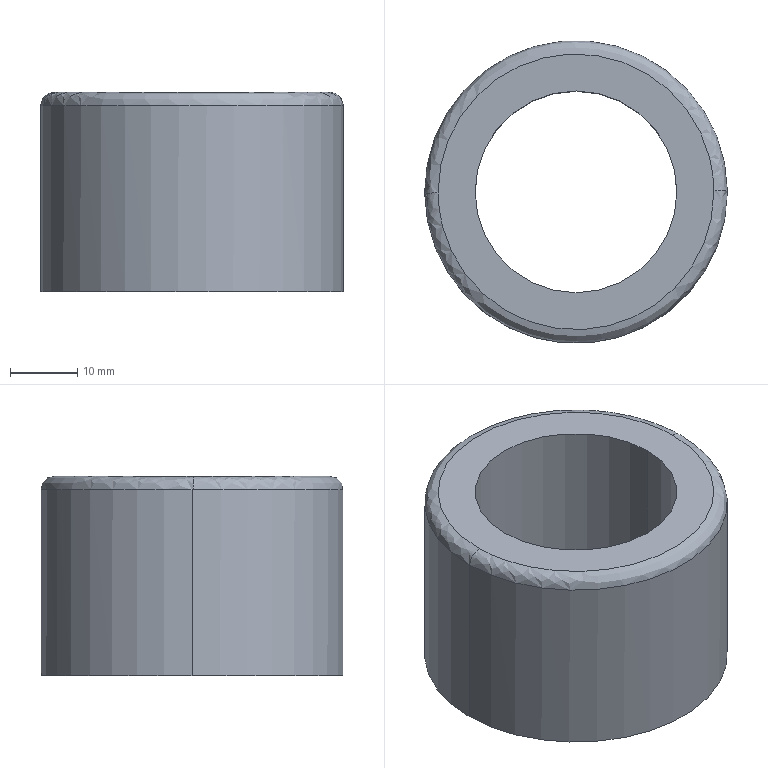Part | SolidWorks | features BaseBody 1 | 1 solid | 8 faces | box 45 x 45 x 29.661 mm | volume 26090 mm3 | cylinder 4 | spline 2 | plane 2 | commonest cylinder face diameters 30 x2 45 x2
STEP:
#1=CARTESIAN_POINT('',(570.036,38.186,21.432));
#2=VERTEX_POINT('',#1);
#3=CARTESIAN_POINT('',(611.034,38.513,21.432));
#4=VERTEX_POINT('',#3);
#5=CARTESIAN_POINT('',(570.036,38.186,21.432));
#6=CARTESIAN_POINT('',(569.708,79.184,21.432));
#7=CARTESIAN_POINT('',(610.707,79.512,21.432));
#8=CARTESIAN_POINT('',(611.034,38.513,21.432));
#9=(BOUNDED_CURVE()B_SPLINE_CURVE(3,(#5,#6,#7,#8),.UNSPECIFIED.,.F.,.T.)B_SPLINE_CURVE_WITH_KNOTS((4,4),(0.,1.),.UNSPECIFIED.)CURVE()GEOMETRIC_REPRESENTATION_ITEM()RATIONAL_B_SPLINE_CURVE((1.,0.3333,0.3333,1.))REPRESENTATION_ITEM(''));
#10=EDGE_CURVE('',#2,#4,#9,.T.);
#11=ORIENTED_EDGE('',*,*,#10,.T.);
#12=CARTESIAN_POINT('',(613.034,38.529,19.432));
#13=VERTEX_POINT('',#12);
#14=CARTESIAN_POINT('',(611.034,38.513,19.432));
#15=DIRECTION('',(-0.007996,1.,0.));
#16=DIRECTION('',(1.,0.007996,-0.000000013));
#17=AXIS2_PLACEMENT_3D('',#14,#15,#16);
#18=CIRCLE('',#17,2.);
#19=EDGE_CURVE('',#4,#13,#18,.T.);
#20=ORIENTED_EDGE('',*,*,#19,.T.);
#21=CARTESIAN_POINT('',(568.035,38.349,19.432));
#22=VERTEX_POINT('',#21);
#23=CARTESIAN_POINT('',(590.535,38.349,19.432));
#24=DIRECTION('',(-0.000000013,0.,-1.));
#25=DIRECTION('',(1.,0.,-0.000000013));
#26=AXIS2_PLACEMENT_3D('',#23,#24,#25);
#27=CIRCLE('',#26,22.5);
#28=EDGE_CURVE('',#22,#13,#27,.T.);
#29=ORIENTED_EDGE('',*,*,#28,.F.);
#30=CARTESIAN_POINT('',(568.036,38.17,19.432));
#31=VERTEX_POINT('',#30);
#32=CARTESIAN_POINT('',(590.535,38.349,19.432));
#33=DIRECTION('',(-0.000000013,0.,-1.));
#34=DIRECTION('',(1.,0.,-0.000000013));
#35=AXIS2_PLACEMENT_3D('',#32,#33,#34);
#36=CIRCLE('',#35,22.5);
#37=EDGE_CURVE('',#31,#22,#36,.T.);
#38=ORIENTED_EDGE('',*,*,#37,.F.);
#39=CARTESIAN_POINT('',(570.036,38.186,19.432));
#40=DIRECTION('',(0.007996,-1.,0.));
#41=DIRECTION('',(-1.,-0.007996,0.000000013));
#42=AXIS2_PLACEMENT_3D('',#39,#40,#41);
#43=CIRCLE('',#42,2.);
#44=EDGE_CURVE('',#2,#31,#43,.T.);
#45=ORIENTED_EDGE('',*,*,#44,.F.);
#46=EDGE_LOOP('',(#11,#20,#29,#38,#45));
#47=FACE_OUTER_BOUND('',#46,.T.);
#48=CARTESIAN_POINT('',(611.034,38.513,21.432));
#49=CARTESIAN_POINT('',(610.707,79.512,21.432));
#50=CARTESIAN_POINT('',(569.708,79.184,21.432));
#51=CARTESIAN_POINT('',(570.036,38.186,21.432));
#52=CARTESIAN_POINT('',(612.206,38.523,21.432));
#53=CARTESIAN_POINT('',(611.859,81.864,21.432));
#54=CARTESIAN_POINT('',(568.518,81.518,21.432));
#55=CARTESIAN_POINT('',(568.864,38.176,21.432));
#56=CARTESIAN_POINT('',(613.034,38.529,20.604));
#57=CARTESIAN_POINT('',(612.675,83.528,20.604));
#58=CARTESIAN_POINT('',(567.676,83.168,20.604));
#59=CARTESIAN_POINT('',(568.036,38.17,20.604));
#60=CARTESIAN_POINT('',(613.034,38.529,19.432));
#61=CARTESIAN_POINT('',(612.675,83.528,19.432));
#62=CARTESIAN_POINT('',(567.676,83.168,19.432));
#63=CARTESIAN_POINT('',(568.036,38.17,19.432));
#64=(BOUNDED_SURFACE()B_SPLINE_SURFACE(3,3,((#48,#49,#50,#51),(#52,#53,#54,#55),(#56,#57,#58,#59),(#60,#61,#62,#63)),.UNSPECIFIED.,.F.,.F.,.F.)B_SPLINE_SURFACE_WITH_KNOTS((4,4),(4,4),(0.,1.),(0.,1.),.UNSPECIFIED.)GEOMETRIC_REPRESENTATION_ITEM()RATIONAL_B_SPLINE_SURFACE(((1.,0.3333,0.3333,1.),(0.8047,0.2682,0.2682,0.8047),(0.8047,0.2682,0.2682,0.8047),(1.,0.3333,0.3333,1.)))REPRESENTATION_ITEM('')SURFACE());
#65=ADVANCED_FACE('',(#47),#64,.T.);
#66=CARTESIAN_POINT('',(613.035,38.349,-8.23));
#67=VERTEX_POINT('',#66);
#68=CARTESIAN_POINT('',(568.035,38.349,-8.23));
#69=VERTEX_POINT('',#68);
#70=CARTESIAN_POINT('',(590.535,38.349,-8.23));
#71=DIRECTION('',(0.000000013,0.,1.));
#72=DIRECTION('',(1.,0.,-0.000000013));
#73=AXIS2_PLACEMENT_3D('',#70,#71,#72);
#74=CIRCLE('',#73,22.5);
#75=EDGE_CURVE('',#67,#69,#74,.T.);
#76=ORIENTED_EDGE('',*,*,#75,.T.);
#77=CARTESIAN_POINT('',(568.035,38.349,6.601));
#78=DIRECTION('',(0.000000013,0.,1.));
#79=VECTOR('',#78,1000.);
#80=LINE('',#77,#79);
#81=EDGE_CURVE('',#69,#22,#80,.T.);
#82=ORIENTED_EDGE('',*,*,#81,.T.);
#83=ORIENTED_EDGE('',*,*,#28,.T.);
#84=CARTESIAN_POINT('',(613.035,38.349,19.432));
#85=VERTEX_POINT('',#84);
#86=CARTESIAN_POINT('',(590.535,38.349,19.432));
#87=DIRECTION('',(-0.000000013,0.,-1.));
#88=DIRECTION('',(1.,0.,-0.000000013));
#89=AXIS2_PLACEMENT_3D('',#86,#87,#88);
#90=CIRCLE('',#89,22.5);
#91=EDGE_CURVE('',#13,#85,#90,.T.);
#92=ORIENTED_EDGE('',*,*,#91,.T.);
#93=CARTESIAN_POINT('',(613.035,38.349,6.601));
#94=DIRECTION('',(0.000000013,0.,1.));
#95=VECTOR('',#94,1000.);
#96=LINE('',#93,#95);
#97=EDGE_CURVE('',#67,#85,#96,.T.);
#98=ORIENTED_EDGE('',*,*,#97,.F.);
#99=EDGE_LOOP('',(#76,#82,#83,#92,#98));
#100=FACE_OUTER_BOUND('',#99,.T.);
#101=CARTESIAN_POINT('',(590.535,38.349,6.601));
#102=DIRECTION('',(0.000000013,0.,1.));
#103=DIRECTION('',(1.,0.,-0.000000013));
#104=AXIS2_PLACEMENT_3D('',#101,#102,#103);
#105=CYLINDRICAL_SURFACE('',#104,22.5);
#106=ADVANCED_FACE('',(#100),#105,.T.);
#107=CARTESIAN_POINT('',(605.535,38.349,21.432));
#108=VERTEX_POINT('',#107);
#109=CARTESIAN_POINT('',(575.535,38.349,21.432));
#110=VERTEX_POINT('',#109);
#111=CARTESIAN_POINT('',(590.535,38.349,21.432));
#112=DIRECTION('',(-0.000000013,0.,-1.));
#113=DIRECTION('',(-1.,0.,0.000000013));
#114=AXIS2_PLACEMENT_3D('',#111,#112,#113);
#115=CIRCLE('',#114,15.);
#116=EDGE_CURVE('',#108,#110,#115,.T.);
#117=ORIENTED_EDGE('',*,*,#116,.F.);
#118=CARTESIAN_POINT('',(605.535,38.349,-8.23));
#119=VERTEX_POINT('',#118);
#120=CARTESIAN_POINT('',(605.535,38.349,21.432));
#121=DIRECTION('',(-0.000000013,0.,-1.));
#122=VECTOR('',#121,1000.);
#123=LINE('',#120,#122);
#124=EDGE_CURVE('',#108,#119,#123,.T.);
#125=ORIENTED_EDGE('',*,*,#124,.T.);
#126=CARTESIAN_POINT('',(575.535,38.349,-8.23));
#127=VERTEX_POINT('',#126);
#128=CARTESIAN_POINT('',(590.535,38.349,-8.23));
#129=DIRECTION('',(0.000000013,0.,1.));
#130=DIRECTION('',(-1.,0.,0.000000013));
#131=AXIS2_PLACEMENT_3D('',#128,#129,#130);
#132=CIRCLE('',#131,15.);
#133=EDGE_CURVE('',#127,#119,#132,.T.);
#134=ORIENTED_EDGE('',*,*,#133,.F.);
#135=CARTESIAN_POINT('',(575.535,38.349,21.432));
#136=DIRECTION('',(-0.000000013,0.,-1.));
#137=VECTOR('',#136,1000.);
#138=LINE('',#135,#137);
#139=EDGE_CURVE('',#110,#127,#138,.T.);
#140=ORIENTED_EDGE('',*,*,#139,.F.);
#141=EDGE_LOOP('',(#117,#125,#134,#140));
#142=FACE_OUTER_BOUND('',#141,.T.);
#143=CARTESIAN_POINT('',(590.535,38.349,21.432));
#144=DIRECTION('',(-0.000000013,0.,-1.));
#145=DIRECTION('',(-1.,0.,0.000000013));
#146=AXIS2_PLACEMENT_3D('',#143,#144,#145);
#147=CYLINDRICAL_SURFACE('',#146,15.);
#148=ADVANCED_FACE('',(#142),#147,.F.);
#149=ORIENTED_EDGE('',*,*,#81,.F.);
#150=CARTESIAN_POINT('',(590.535,38.349,-8.23));
#151=DIRECTION('',(0.000000013,0.,1.));
#152=DIRECTION('',(1.,0.,-0.000000013));
#153=AXIS2_PLACEMENT_3D('',#150,#151,#152);
#154=CIRCLE('',#153,22.5);
#155=EDGE_CURVE('',#69,#67,#154,.T.);
#156=ORIENTED_EDGE('',*,*,#155,.T.);
#157=ORIENTED_EDGE('',*,*,#97,.T.);
#158=CARTESIAN_POINT('',(590.535,38.349,19.432));
#159=DIRECTION('',(-0.000000013,0.,-1.));
#160=DIRECTION('',(1.,0.,-0.000000013));
#161=AXIS2_PLACEMENT_3D('',#158,#159,#160);
#162=CIRCLE('',#161,22.5);
#163=EDGE_CURVE('',#85,#31,#162,.T.);
#164=ORIENTED_EDGE('',*,*,#163,.T.);
#165=ORIENTED_EDGE('',*,*,#37,.T.);
#166=EDGE_LOOP('',(#149,#156,#157,#164,#165));
#167=FACE_OUTER_BOUND('',#166,.T.);
#168=CARTESIAN_POINT('',(590.535,38.349,6.601));
#169=DIRECTION('',(0.000000013,0.,1.));
#170=DIRECTION('',(1.,0.,-0.000000013));
#171=AXIS2_PLACEMENT_3D('',#168,#169,#170);
#172=CYLINDRICAL_SURFACE('',#171,22.5);
#173=ADVANCED_FACE('',(#167),#172,.T.);
#174=ORIENTED_EDGE('',*,*,#75,.F.);
#175=ORIENTED_EDGE('',*,*,#155,.F.);
#176=EDGE_LOOP('',(#174,#175));
#177=FACE_OUTER_BOUND('',#176,.T.);
#178=ORIENTED_EDGE('',*,*,#133,.T.);
#179=CARTESIAN_POINT('',(590.535,38.349,-8.23));
#180=DIRECTION('',(0.000000013,0.,1.));
#181=DIRECTION('',(-1.,0.,0.000000013));
#182=AXIS2_PLACEMENT_3D('',#179,#180,#181);
#183=CIRCLE('',#182,15.);
#184=EDGE_CURVE('',#119,#127,#183,.T.);
#185=ORIENTED_EDGE('',*,*,#184,.T.);
#186=EDGE_LOOP('',(#178,#185));
#187=FACE_BOUND('',#186,.T.);
#188=CARTESIAN_POINT('',(601.785,38.439,-8.23));
#189=DIRECTION('',(-0.000000013,0.,-1.));
#190=DIRECTION('',(-1.,0.,0.000000013));
#191=AXIS2_PLACEMENT_3D('',#188,#189,#190);
#192=PLANE('',#191);
#193=ADVANCED_FACE('',(#177,#187),#192,.T.);
#194=ORIENTED_EDGE('',*,*,#19,.F.);
#195=CARTESIAN_POINT('',(611.034,38.513,21.432));
#196=CARTESIAN_POINT('',(611.362,-2.485,21.432));
#197=CARTESIAN_POINT('',(570.364,-2.813,21.432));
#198=CARTESIAN_POINT('',(570.036,38.186,21.432));
#199=(BOUNDED_CURVE()B_SPLINE_CURVE(3,(#195,#196,#197,#198),.UNSPECIFIED.,.F.,.T.)B_SPLINE_CURVE_WITH_KNOTS((4,4),(0.,1.),.UNSPECIFIED.)CURVE()GEOMETRIC_REPRESENTATION_ITEM()RATIONAL_B_SPLINE_CURVE((1.,0.3333,0.3333,1.))REPRESENTATION_ITEM(''));
#200=EDGE_CURVE('',#4,#2,#199,.T.);
#201=ORIENTED_EDGE('',*,*,#200,.T.);
#202=ORIENTED_EDGE('',*,*,#44,.T.);
#203=ORIENTED_EDGE('',*,*,#163,.F.);
#204=ORIENTED_EDGE('',*,*,#91,.F.);
#205=EDGE_LOOP('',(#194,#201,#202,#203,#204));
#206=FACE_OUTER_BOUND('',#205,.T.);
#207=CARTESIAN_POINT('',(570.036,38.186,21.432));
#208=CARTESIAN_POINT('',(570.364,-2.813,21.432));
#209=CARTESIAN_POINT('',(611.362,-2.485,21.432));
#210=CARTESIAN_POINT('',(611.034,38.513,21.432));
#211=CARTESIAN_POINT('',(568.864,38.176,21.432));
#212=CARTESIAN_POINT('',(569.211,-5.166,21.432));
#213=CARTESIAN_POINT('',(612.553,-4.819,21.432));
#214=CARTESIAN_POINT('',(612.206,38.523,21.432));
#215=CARTESIAN_POINT('',(568.036,38.17,20.604));
#216=CARTESIAN_POINT('',(568.396,-6.829,20.604));
#217=CARTESIAN_POINT('',(613.394,-6.469,20.604));
#218=CARTESIAN_POINT('',(613.034,38.529,20.604));
#219=CARTESIAN_POINT('',(568.036,38.17,19.432));
#220=CARTESIAN_POINT('',(568.396,-6.829,19.432));
#221=CARTESIAN_POINT('',(613.394,-6.469,19.432));
#222=CARTESIAN_POINT('',(613.034,38.529,19.432));
#223=(BOUNDED_SURFACE()B_SPLINE_SURFACE(3,3,((#207,#208,#209,#210),(#211,#212,#213,#214),(#215,#216,#217,#218),(#219,#220,#221,#222)),.UNSPECIFIED.,.F.,.F.,.F.)B_SPLINE_SURFACE_WITH_KNOTS((4,4),(4,4),(0.,1.),(0.,1.),.UNSPECIFIED.)GEOMETRIC_REPRESENTATION_ITEM()RATIONAL_B_SPLINE_SURFACE(((1.,0.3333,0.3333,1.),(0.8047,0.2682,0.2682,0.8047),(0.8047,0.2682,0.2682,0.8047),(1.,0.3333,0.3333,1.)))REPRESENTATION_ITEM('')SURFACE());
#224=ADVANCED_FACE('',(#206),#223,.T.);
#225=ORIENTED_EDGE('',*,*,#124,.F.);
#226=CARTESIAN_POINT('',(590.535,38.349,21.432));
#227=DIRECTION('',(-0.000000013,0.,-1.));
#228=DIRECTION('',(-1.,0.,0.000000013));
#229=AXIS2_PLACEMENT_3D('',#226,#227,#228);
#230=CIRCLE('',#229,15.);
#231=EDGE_CURVE('',#110,#108,#230,.T.);
#232=ORIENTED_EDGE('',*,*,#231,.F.);
#233=ORIENTED_EDGE('',*,*,#139,.T.);
#234=ORIENTED_EDGE('',*,*,#184,.F.);
#235=EDGE_LOOP('',(#225,#232,#233,#234));
#236=FACE_OUTER_BOUND('',#235,.T.);
#237=CARTESIAN_POINT('',(590.535,38.349,21.432));
#238=DIRECTION('',(-0.000000013,0.,-1.));
#239=DIRECTION('',(-1.,0.,0.000000013));
#240=AXIS2_PLACEMENT_3D('',#237,#238,#239);
#241=CYLINDRICAL_SURFACE('',#240,15.);
#242=ADVANCED_FACE('',(#236),#241,.F.);
#243=ORIENTED_EDGE('',*,*,#200,.F.);
#244=ORIENTED_EDGE('',*,*,#10,.F.);
#245=EDGE_LOOP('',(#243,#244));
#246=FACE_OUTER_BOUND('',#245,.T.);
#247=ORIENTED_EDGE('',*,*,#231,.T.);
#248=ORIENTED_EDGE('',*,*,#116,.T.);
#249=EDGE_LOOP('',(#247,#248));
#250=FACE_BOUND('',#249,.T.);
#251=CARTESIAN_POINT('',(601.785,38.439,21.432));
#252=DIRECTION('',(0.000000013,0.,1.));
#253=DIRECTION('',(1.,0.,-0.000000013));
#254=AXIS2_PLACEMENT_3D('',#251,#252,#253);
#255=PLANE('',#254);
#256=ADVANCED_FACE('',(#246,#250),#255,.T.);
#257=CLOSED_SHELL('',(#65,#106,#148,#173,#193,#224,#242,#256));
#258=MANIFOLD_SOLID_BREP('',#257);
#259=CARTESIAN_POINT('',(0.,0.,0.));
#260=DIRECTION('',(0.,0.,1.));
#261=DIRECTION('',(1.,0.,0.));
#262=AXIS2_PLACEMENT_3D('',#259,#260,#261);
#263=(LENGTH_UNIT()NAMED_UNIT(*)SI_UNIT(.MILLI.,.METRE.));
#264=UNCERTAINTY_MEASURE_WITH_UNIT(LENGTH_MEASURE(0.00001),#263,'','');
#265=(NAMED_UNIT(*)PLANE_ANGLE_UNIT()SI_UNIT($,.RADIAN.));
#266=(NAMED_UNIT(*)SI_UNIT($,.STERADIAN.)SOLID_ANGLE_UNIT());
#267=(GEOMETRIC_REPRESENTATION_CONTEXT(3)GLOBAL_UNCERTAINTY_ASSIGNED_CONTEXT((#264))GLOBAL_UNIT_ASSIGNED_CONTEXT((#263,#265,#266))REPRESENTATION_CONTEXT('',''));
#268=ADVANCED_BREP_SHAPE_REPRESENTATION('',(#258,#262),#267);